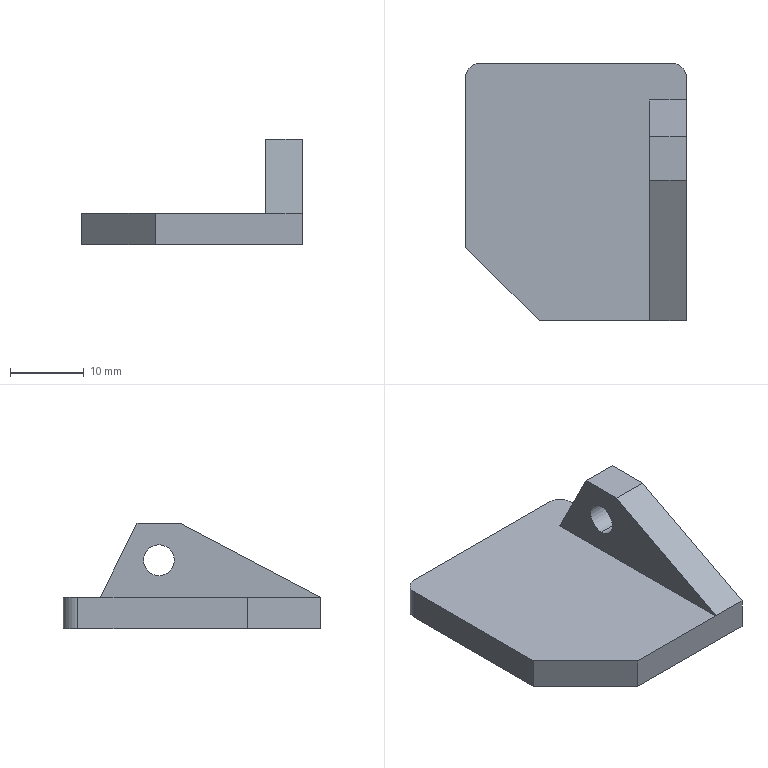Part | SolidWorks | features BaseBody 1 | 1 solid | 15 faces | box 30 x 35 x 14.3 mm | volume 5075 mm3 | plane 11 | cylinder 4 | commonest cylinder face diameters 4 x2 4.2 x2
STEP:
#1=CARTESIAN_POINT('',(269.946,-4053.971,2158.071));
#2=VERTEX_POINT('',#1);
#3=CARTESIAN_POINT('',(269.946,-4053.971,2153.871));
#4=VERTEX_POINT('',#3);
#5=CARTESIAN_POINT('',(269.946,-4053.971,2155.971));
#6=DIRECTION('',(1.,0.,0.));
#7=DIRECTION('',(0.,0.,-1.));
#8=AXIS2_PLACEMENT_3D('',#5,#6,#7);
#9=CIRCLE('',#8,2.1);
#10=EDGE_CURVE('',#2,#4,#9,.T.);
#11=ORIENTED_EDGE('',*,*,#10,.F.);
#12=CARTESIAN_POINT('',(274.946,-4053.971,2158.071));
#13=VERTEX_POINT('',#12);
#14=CARTESIAN_POINT('',(274.946,-4053.971,2158.071));
#15=DIRECTION('',(1.,0.,0.));
#16=VECTOR('',#15,1000.);
#17=LINE('',#14,#16);
#18=EDGE_CURVE('',#2,#13,#17,.T.);
#19=ORIENTED_EDGE('',*,*,#18,.T.);
#20=CARTESIAN_POINT('',(274.946,-4053.971,2153.871));
#21=VERTEX_POINT('',#20);
#22=CARTESIAN_POINT('',(274.946,-4053.971,2155.971));
#23=DIRECTION('',(-1.,0.,0.));
#24=DIRECTION('',(0.,0.,-1.));
#25=AXIS2_PLACEMENT_3D('',#22,#23,#24);
#26=CIRCLE('',#25,2.1);
#27=EDGE_CURVE('',#21,#13,#26,.T.);
#28=ORIENTED_EDGE('',*,*,#27,.F.);
#29=CARTESIAN_POINT('',(274.946,-4053.971,2153.871));
#30=DIRECTION('',(1.,0.,0.));
#31=VECTOR('',#30,1000.);
#32=LINE('',#29,#31);
#33=EDGE_CURVE('',#4,#21,#32,.T.);
#34=ORIENTED_EDGE('',*,*,#33,.F.);
#35=EDGE_LOOP('',(#11,#19,#28,#34));
#36=FACE_OUTER_BOUND('',#35,.T.);
#37=CARTESIAN_POINT('',(274.946,-4053.971,2155.971));
#38=DIRECTION('',(1.,0.,0.));
#39=DIRECTION('',(0.,0.,-1.));
#40=AXIS2_PLACEMENT_3D('',#37,#38,#39);
#41=CYLINDRICAL_SURFACE('',#40,2.1);
#42=ADVANCED_FACE('',(#36),#41,.F.);
#43=CARTESIAN_POINT('',(272.946,-4040.971,2146.671));
#44=VERTEX_POINT('',#43);
#45=CARTESIAN_POINT('',(246.946,-4040.971,2146.671));
#46=VERTEX_POINT('',#45);
#47=CARTESIAN_POINT('',(254.946,-4040.971,2146.671));
#48=DIRECTION('',(-1.,0.,0.));
#49=VECTOR('',#48,1000.);
#50=LINE('',#47,#49);
#51=EDGE_CURVE('',#44,#46,#50,.T.);
#52=ORIENTED_EDGE('',*,*,#51,.F.);
#53=CARTESIAN_POINT('',(274.946,-4042.971,2146.671));
#54=VERTEX_POINT('',#53);
#55=CARTESIAN_POINT('',(272.946,-4042.971,2146.671));
#56=DIRECTION('',(0.,0.,1.));
#57=DIRECTION('',(1.,0.,0.));
#58=AXIS2_PLACEMENT_3D('',#55,#56,#57);
#59=CIRCLE('',#58,2.);
#60=EDGE_CURVE('',#54,#44,#59,.T.);
#61=ORIENTED_EDGE('',*,*,#60,.F.);
#62=CARTESIAN_POINT('',(274.946,-4075.971,2146.671));
#63=VERTEX_POINT('',#62);
#64=CARTESIAN_POINT('',(274.946,-4075.971,2146.671));
#65=DIRECTION('',(0.,1.,0.));
#66=VECTOR('',#65,1000.);
#67=LINE('',#64,#66);
#68=EDGE_CURVE('',#63,#54,#67,.T.);
#69=ORIENTED_EDGE('',*,*,#68,.F.);
#70=CARTESIAN_POINT('',(254.946,-4075.971,2146.671));
#71=VERTEX_POINT('',#70);
#72=CARTESIAN_POINT('',(254.946,-4075.971,2146.671));
#73=DIRECTION('',(1.,0.,0.));
#74=VECTOR('',#73,1000.);
#75=LINE('',#72,#74);
#76=EDGE_CURVE('',#71,#63,#75,.T.);
#77=ORIENTED_EDGE('',*,*,#76,.F.);
#78=CARTESIAN_POINT('',(244.946,-4065.971,2146.671));
#79=VERTEX_POINT('',#78);
#80=CARTESIAN_POINT('',(244.946,-4065.971,2146.671));
#81=DIRECTION('',(0.7071,-0.7071,0.));
#82=VECTOR('',#81,1000.);
#83=LINE('',#80,#82);
#84=EDGE_CURVE('',#79,#71,#83,.T.);
#85=ORIENTED_EDGE('',*,*,#84,.F.);
#86=CARTESIAN_POINT('',(244.946,-4042.971,2146.671));
#87=VERTEX_POINT('',#86);
#88=CARTESIAN_POINT('',(244.946,-4075.971,2146.671));
#89=DIRECTION('',(0.,-1.,0.));
#90=VECTOR('',#89,1000.);
#91=LINE('',#88,#90);
#92=EDGE_CURVE('',#87,#79,#91,.T.);
#93=ORIENTED_EDGE('',*,*,#92,.F.);
#94=CARTESIAN_POINT('',(246.946,-4042.971,2146.671));
#95=DIRECTION('',(0.,0.,1.));
#96=DIRECTION('',(1.,0.,0.));
#97=AXIS2_PLACEMENT_3D('',#94,#95,#96);
#98=CIRCLE('',#97,2.);
#99=EDGE_CURVE('',#46,#87,#98,.T.);
#100=ORIENTED_EDGE('',*,*,#99,.F.);
#101=EDGE_LOOP('',(#52,#61,#69,#77,#85,#93,#100));
#102=FACE_OUTER_BOUND('',#101,.T.);
#103=CARTESIAN_POINT('',(254.946,-4075.971,2146.671));
#104=DIRECTION('',(0.,0.,1.));
#105=DIRECTION('',(0.,-1.,0.));
#106=AXIS2_PLACEMENT_3D('',#103,#104,#105);
#107=PLANE('',#106);
#108=ADVANCED_FACE('',(#102),#107,.F.);
#109=CARTESIAN_POINT('',(244.946,-4042.971,2150.921));
#110=VERTEX_POINT('',#109);
#111=CARTESIAN_POINT('',(244.946,-4042.971,2150.921));
#112=DIRECTION('',(0.,0.,1.));
#113=VECTOR('',#112,1000.);
#114=LINE('',#111,#113);
#115=EDGE_CURVE('',#87,#110,#114,.T.);
#116=ORIENTED_EDGE('',*,*,#115,.T.);
#117=CARTESIAN_POINT('',(246.946,-4040.971,2150.921));
#118=VERTEX_POINT('',#117);
#119=CARTESIAN_POINT('',(246.946,-4042.971,2150.921));
#120=DIRECTION('',(0.,0.,-1.));
#121=DIRECTION('',(1.,0.,0.));
#122=AXIS2_PLACEMENT_3D('',#119,#120,#121);
#123=CIRCLE('',#122,2.);
#124=EDGE_CURVE('',#110,#118,#123,.T.);
#125=ORIENTED_EDGE('',*,*,#124,.T.);
#126=CARTESIAN_POINT('',(246.946,-4040.971,2150.921));
#127=DIRECTION('',(0.,0.,-1.));
#128=VECTOR('',#127,1000.);
#129=LINE('',#126,#128);
#130=EDGE_CURVE('',#118,#46,#129,.T.);
#131=ORIENTED_EDGE('',*,*,#130,.T.);
#132=ORIENTED_EDGE('',*,*,#99,.T.);
#133=EDGE_LOOP('',(#116,#125,#131,#132));
#134=FACE_OUTER_BOUND('',#133,.T.);
#135=CARTESIAN_POINT('',(246.946,-4042.971,2150.921));
#136=DIRECTION('',(0.,0.,1.));
#137=DIRECTION('',(1.,0.,0.));
#138=AXIS2_PLACEMENT_3D('',#135,#136,#137);
#139=CYLINDRICAL_SURFACE('',#138,2.);
#140=ADVANCED_FACE('',(#134),#139,.T.);
#141=ORIENTED_EDGE('',*,*,#130,.F.);
#142=CARTESIAN_POINT('',(272.946,-4040.971,2150.921));
#143=VERTEX_POINT('',#142);
#144=CARTESIAN_POINT('',(244.946,-4040.971,2150.921));
#145=DIRECTION('',(1.,0.,0.));
#146=VECTOR('',#145,1000.);
#147=LINE('',#144,#146);
#148=EDGE_CURVE('',#118,#143,#147,.T.);
#149=ORIENTED_EDGE('',*,*,#148,.T.);
#150=CARTESIAN_POINT('',(272.946,-4040.971,2150.921));
#151=DIRECTION('',(0.,0.,-1.));
#152=VECTOR('',#151,1000.);
#153=LINE('',#150,#152);
#154=EDGE_CURVE('',#143,#44,#153,.T.);
#155=ORIENTED_EDGE('',*,*,#154,.T.);
#156=ORIENTED_EDGE('',*,*,#51,.T.);
#157=EDGE_LOOP('',(#141,#149,#155,#156));
#158=FACE_OUTER_BOUND('',#157,.T.);
#159=CARTESIAN_POINT('',(244.946,-4040.971,2150.921));
#160=DIRECTION('',(0.,1.,0.));
#161=DIRECTION('',(0.,0.,1.));
#162=AXIS2_PLACEMENT_3D('',#159,#160,#161);
#163=PLANE('',#162);
#164=ADVANCED_FACE('',(#158),#163,.T.);
#165=ORIENTED_EDGE('',*,*,#154,.F.);
#166=CARTESIAN_POINT('',(274.946,-4042.971,2150.921));
#167=VERTEX_POINT('',#166);
#168=CARTESIAN_POINT('',(272.946,-4042.971,2150.921));
#169=DIRECTION('',(0.,0.,-1.));
#170=DIRECTION('',(1.,0.,0.));
#171=AXIS2_PLACEMENT_3D('',#168,#169,#170);
#172=CIRCLE('',#171,2.);
#173=EDGE_CURVE('',#143,#167,#172,.T.);
#174=ORIENTED_EDGE('',*,*,#173,.T.);
#175=CARTESIAN_POINT('',(274.946,-4042.971,2150.921));
#176=DIRECTION('',(0.,0.,-1.));
#177=VECTOR('',#176,1000.);
#178=LINE('',#175,#177);
#179=EDGE_CURVE('',#167,#54,#178,.T.);
#180=ORIENTED_EDGE('',*,*,#179,.T.);
#181=ORIENTED_EDGE('',*,*,#60,.T.);
#182=EDGE_LOOP('',(#165,#174,#180,#181));
#183=FACE_OUTER_BOUND('',#182,.T.);
#184=CARTESIAN_POINT('',(272.946,-4042.971,2150.921));
#185=DIRECTION('',(0.,0.,1.));
#186=DIRECTION('',(1.,0.,0.));
#187=AXIS2_PLACEMENT_3D('',#184,#185,#186);
#188=CYLINDRICAL_SURFACE('',#187,2.);
#189=ADVANCED_FACE('',(#183),#188,.T.);
#190=CARTESIAN_POINT('',(274.946,-4075.971,2150.921));
#191=VERTEX_POINT('',#190);
#192=CARTESIAN_POINT('',(274.946,-4075.971,2150.921));
#193=DIRECTION('',(0.,0.,-1.));
#194=VECTOR('',#193,1000.);
#195=LINE('',#192,#194);
#196=EDGE_CURVE('',#191,#63,#195,.T.);
#197=ORIENTED_EDGE('',*,*,#196,.T.);
#198=ORIENTED_EDGE('',*,*,#68,.T.);
#199=ORIENTED_EDGE('',*,*,#179,.F.);
#200=CARTESIAN_POINT('',(274.946,-4045.971,2150.921));
#201=VERTEX_POINT('',#200);
#202=CARTESIAN_POINT('',(274.946,-4040.971,2150.921));
#203=DIRECTION('',(0.,-1.,0.));
#204=VECTOR('',#203,1000.);
#205=LINE('',#202,#204);
#206=EDGE_CURVE('',#167,#201,#205,.T.);
#207=ORIENTED_EDGE('',*,*,#206,.T.);
#208=CARTESIAN_POINT('',(274.946,-4050.996,2160.971));
#209=VERTEX_POINT('',#208);
#210=CARTESIAN_POINT('',(274.946,-4045.971,2150.921));
#211=DIRECTION('',(0.,-0.4472,0.8944));
#212=VECTOR('',#211,1000.);
#213=LINE('',#210,#212);
#214=EDGE_CURVE('',#201,#209,#213,.T.);
#215=ORIENTED_EDGE('',*,*,#214,.T.);
#216=CARTESIAN_POINT('',(274.946,-4056.876,2160.971));
#217=VERTEX_POINT('',#216);
#218=CARTESIAN_POINT('',(274.946,-4040.971,2160.971));
#219=DIRECTION('',(0.,-1.,0.));
#220=VECTOR('',#219,1000.);
#221=LINE('',#218,#220);
#222=EDGE_CURVE('',#209,#217,#221,.T.);
#223=ORIENTED_EDGE('',*,*,#222,.T.);
#224=CARTESIAN_POINT('',(274.946,-4056.876,2160.971));
#225=DIRECTION('',(0.,-0.8849,-0.4657));
#226=VECTOR('',#225,1000.);
#227=LINE('',#224,#226);
#228=EDGE_CURVE('',#217,#191,#227,.T.);
#229=ORIENTED_EDGE('',*,*,#228,.T.);
#230=EDGE_LOOP('',(#197,#198,#199,#207,#215,#223,#229));
#231=FACE_OUTER_BOUND('',#230,.T.);
#232=ORIENTED_EDGE('',*,*,#27,.T.);
#233=CARTESIAN_POINT('',(274.946,-4053.971,2155.971));
#234=DIRECTION('',(-1.,0.,0.));
#235=DIRECTION('',(0.,0.,-1.));
#236=AXIS2_PLACEMENT_3D('',#233,#234,#235);
#237=CIRCLE('',#236,2.1);
#238=EDGE_CURVE('',#13,#21,#237,.T.);
#239=ORIENTED_EDGE('',*,*,#238,.T.);
#240=EDGE_LOOP('',(#232,#239));
#241=FACE_BOUND('',#240,.T.);
#242=CARTESIAN_POINT('',(274.946,-4040.971,2150.921));
#243=DIRECTION('',(1.,0.,0.));
#244=DIRECTION('',(0.,1.,0.));
#245=AXIS2_PLACEMENT_3D('',#242,#243,#244);
#246=PLANE('',#245);
#247=ADVANCED_FACE('',(#231,#241),#246,.T.);
#248=CARTESIAN_POINT('',(269.946,-4075.971,2150.921));
#249=VERTEX_POINT('',#248);
#250=CARTESIAN_POINT('',(274.946,-4075.971,2150.921));
#251=DIRECTION('',(-1.,0.,0.));
#252=VECTOR('',#251,1000.);
#253=LINE('',#250,#252);
#254=EDGE_CURVE('',#191,#249,#253,.T.);
#255=ORIENTED_EDGE('',*,*,#254,.T.);
#256=CARTESIAN_POINT('',(254.946,-4075.971,2150.921));
#257=VERTEX_POINT('',#256);
#258=CARTESIAN_POINT('',(274.946,-4075.971,2150.921));
#259=DIRECTION('',(-1.,0.,0.));
#260=VECTOR('',#259,1000.);
#261=LINE('',#258,#260);
#262=EDGE_CURVE('',#249,#257,#261,.T.);
#263=ORIENTED_EDGE('',*,*,#262,.T.);
#264=CARTESIAN_POINT('',(254.946,-4075.971,2150.921));
#265=DIRECTION('',(0.,0.,-1.));
#266=VECTOR('',#265,1000.);
#267=LINE('',#264,#266);
#268=EDGE_CURVE('',#257,#71,#267,.T.);
#269=ORIENTED_EDGE('',*,*,#268,.T.);
#270=ORIENTED_EDGE('',*,*,#76,.T.);
#271=ORIENTED_EDGE('',*,*,#196,.F.);
#272=EDGE_LOOP('',(#255,#263,#269,#270,#271));
#273=FACE_OUTER_BOUND('',#272,.T.);
#274=CARTESIAN_POINT('',(274.946,-4075.971,2150.921));
#275=DIRECTION('',(0.,-1.,0.));
#276=DIRECTION('',(0.,0.,-1.));
#277=AXIS2_PLACEMENT_3D('',#274,#275,#276);
#278=PLANE('',#277);
#279=ADVANCED_FACE('',(#273),#278,.T.);
#280=ORIENTED_EDGE('',*,*,#268,.F.);
#281=CARTESIAN_POINT('',(244.946,-4065.971,2150.921));
#282=VERTEX_POINT('',#281);
#283=CARTESIAN_POINT('',(254.946,-4075.971,2150.921));
#284=DIRECTION('',(-0.7071,0.7071,0.));
#285=VECTOR('',#284,1000.);
#286=LINE('',#283,#285);
#287=EDGE_CURVE('',#257,#282,#286,.T.);
#288=ORIENTED_EDGE('',*,*,#287,.T.);
#289=CARTESIAN_POINT('',(244.946,-4065.971,2150.921));
#290=DIRECTION('',(0.,0.,-1.));
#291=VECTOR('',#290,1000.);
#292=LINE('',#289,#291);
#293=EDGE_CURVE('',#282,#79,#292,.T.);
#294=ORIENTED_EDGE('',*,*,#293,.T.);
#295=ORIENTED_EDGE('',*,*,#84,.T.);
#296=EDGE_LOOP('',(#280,#288,#294,#295));
#297=FACE_OUTER_BOUND('',#296,.T.);
#298=CARTESIAN_POINT('',(254.946,-4075.971,2150.921));
#299=DIRECTION('',(-0.7071,-0.7071,0.));
#300=DIRECTION('',(0.7071,-0.7071,0.));
#301=AXIS2_PLACEMENT_3D('',#298,#299,#300);
#302=PLANE('',#301);
#303=ADVANCED_FACE('',(#297),#302,.T.);
#304=ORIENTED_EDGE('',*,*,#293,.F.);
#305=CARTESIAN_POINT('',(244.946,-4065.971,2150.921));
#306=DIRECTION('',(0.,1.,0.));
#307=VECTOR('',#306,1000.);
#308=LINE('',#305,#307);
#309=EDGE_CURVE('',#282,#110,#308,.T.);
#310=ORIENTED_EDGE('',*,*,#309,.T.);
#311=ORIENTED_EDGE('',*,*,#115,.F.);
#312=ORIENTED_EDGE('',*,*,#92,.T.);
#313=EDGE_LOOP('',(#304,#310,#311,#312));
#314=FACE_OUTER_BOUND('',#313,.T.);
#315=CARTESIAN_POINT('',(244.946,-4065.971,2150.921));
#316=DIRECTION('',(-1.,0.,0.));
#317=DIRECTION('',(0.,-1.,0.));
#318=AXIS2_PLACEMENT_3D('',#315,#316,#317);
#319=PLANE('',#318);
#320=ADVANCED_FACE('',(#314),#319,.T.);
#321=ORIENTED_EDGE('',*,*,#287,.F.);
#322=ORIENTED_EDGE('',*,*,#262,.F.);
#323=CARTESIAN_POINT('',(269.946,-4045.971,2150.921));
#324=VERTEX_POINT('',#323);
#325=CARTESIAN_POINT('',(269.946,-4059.971,2150.921));
#326=DIRECTION('',(0.,1.,0.));
#327=VECTOR('',#326,1000.);
#328=LINE('',#325,#327);
#329=EDGE_CURVE('',#249,#324,#328,.T.);
#330=ORIENTED_EDGE('',*,*,#329,.T.);
#331=CARTESIAN_POINT('',(258.946,-4045.971,2150.921));
#332=DIRECTION('',(1.,0.,0.));
#333=VECTOR('',#332,1000.);
#334=LINE('',#331,#333);
#335=EDGE_CURVE('',#324,#201,#334,.T.);
#336=ORIENTED_EDGE('',*,*,#335,.T.);
#337=ORIENTED_EDGE('',*,*,#206,.F.);
#338=ORIENTED_EDGE('',*,*,#173,.F.);
#339=ORIENTED_EDGE('',*,*,#148,.F.);
#340=ORIENTED_EDGE('',*,*,#124,.F.);
#341=ORIENTED_EDGE('',*,*,#309,.F.);
#342=EDGE_LOOP('',(#321,#322,#330,#336,#337,#338,#339,#340,#341));
#343=FACE_OUTER_BOUND('',#342,.T.);
#344=CARTESIAN_POINT('',(258.946,-4059.971,2150.921));
#345=DIRECTION('',(0.,0.,1.));
#346=DIRECTION('',(0.,-1.,0.));
#347=AXIS2_PLACEMENT_3D('',#344,#345,#346);
#348=PLANE('',#347);
#349=ADVANCED_FACE('',(#343),#348,.T.);
#350=ORIENTED_EDGE('',*,*,#228,.F.);
#351=CARTESIAN_POINT('',(269.946,-4056.876,2160.971));
#352=VERTEX_POINT('',#351);
#353=CARTESIAN_POINT('',(274.946,-4056.876,2160.971));
#354=DIRECTION('',(-1.,0.,0.));
#355=VECTOR('',#354,1000.);
#356=LINE('',#353,#355);
#357=EDGE_CURVE('',#217,#352,#356,.T.);
#358=ORIENTED_EDGE('',*,*,#357,.T.);
#359=CARTESIAN_POINT('',(269.946,-4075.971,2150.921));
#360=DIRECTION('',(0.,-0.8849,-0.4657));
#361=VECTOR('',#360,1000.);
#362=LINE('',#359,#361);
#363=EDGE_CURVE('',#352,#249,#362,.T.);
#364=ORIENTED_EDGE('',*,*,#363,.T.);
#365=ORIENTED_EDGE('',*,*,#254,.F.);
#366=EDGE_LOOP('',(#350,#358,#364,#365));
#367=FACE_OUTER_BOUND('',#366,.T.);
#368=CARTESIAN_POINT('',(274.946,-4075.971,2150.921));
#369=DIRECTION('',(0.,-0.4657,0.8849));
#370=DIRECTION('',(0.,-0.8849,-0.4657));
#371=AXIS2_PLACEMENT_3D('',#368,#369,#370);
#372=PLANE('',#371);
#373=ADVANCED_FACE('',(#367),#372,.T.);
#374=ORIENTED_EDGE('',*,*,#222,.F.);
#375=CARTESIAN_POINT('',(269.946,-4050.996,2160.971));
#376=VERTEX_POINT('',#375);
#377=CARTESIAN_POINT('',(274.946,-4050.996,2160.971));
#378=DIRECTION('',(-1.,0.,0.));
#379=VECTOR('',#378,1000.);
#380=LINE('',#377,#379);
#381=EDGE_CURVE('',#209,#376,#380,.T.);
#382=ORIENTED_EDGE('',*,*,#381,.T.);
#383=CARTESIAN_POINT('',(269.946,-4056.971,2160.971));
#384=DIRECTION('',(0.,-1.,0.));
#385=VECTOR('',#384,1000.);
#386=LINE('',#383,#385);
#387=EDGE_CURVE('',#376,#352,#386,.T.);
#388=ORIENTED_EDGE('',*,*,#387,.T.);
#389=ORIENTED_EDGE('',*,*,#357,.F.);
#390=EDGE_LOOP('',(#374,#382,#388,#389));
#391=FACE_OUTER_BOUND('',#390,.T.);
#392=CARTESIAN_POINT('',(274.946,-4056.971,2160.971));
#393=DIRECTION('',(0.,0.,1.));
#394=DIRECTION('',(0.,-1.,0.));
#395=AXIS2_PLACEMENT_3D('',#392,#393,#394);
#396=PLANE('',#395);
#397=ADVANCED_FACE('',(#391),#396,.T.);
#398=ORIENTED_EDGE('',*,*,#214,.F.);
#399=ORIENTED_EDGE('',*,*,#335,.F.);
#400=CARTESIAN_POINT('',(269.946,-4050.971,2160.921));
#401=DIRECTION('',(0.,-0.4472,0.8944));
#402=VECTOR('',#401,1000.);
#403=LINE('',#400,#402);
#404=EDGE_CURVE('',#324,#376,#403,.T.);
#405=ORIENTED_EDGE('',*,*,#404,.T.);
#406=ORIENTED_EDGE('',*,*,#381,.F.);
#407=EDGE_LOOP('',(#398,#399,#405,#406));
#408=FACE_OUTER_BOUND('',#407,.T.);
#409=CARTESIAN_POINT('',(274.946,-4050.971,2160.921));
#410=DIRECTION('',(0.,0.8944,0.4472));
#411=DIRECTION('',(0.,-0.4472,0.8944));
#412=AXIS2_PLACEMENT_3D('',#409,#410,#411);
#413=PLANE('',#412);
#414=ADVANCED_FACE('',(#408),#413,.T.);
#415=ORIENTED_EDGE('',*,*,#18,.F.);
#416=CARTESIAN_POINT('',(269.946,-4053.971,2155.971));
#417=DIRECTION('',(1.,0.,0.));
#418=DIRECTION('',(0.,0.,-1.));
#419=AXIS2_PLACEMENT_3D('',#416,#417,#418);
#420=CIRCLE('',#419,2.1);
#421=EDGE_CURVE('',#4,#2,#420,.T.);
#422=ORIENTED_EDGE('',*,*,#421,.F.);
#423=ORIENTED_EDGE('',*,*,#33,.T.);
#424=ORIENTED_EDGE('',*,*,#238,.F.);
#425=EDGE_LOOP('',(#415,#422,#423,#424));
#426=FACE_OUTER_BOUND('',#425,.T.);
#427=CARTESIAN_POINT('',(274.946,-4053.971,2155.971));
#428=DIRECTION('',(1.,0.,0.));
#429=DIRECTION('',(0.,0.,-1.));
#430=AXIS2_PLACEMENT_3D('',#427,#428,#429);
#431=CYLINDRICAL_SURFACE('',#430,2.1);
#432=ADVANCED_FACE('',(#426),#431,.F.);
#433=ORIENTED_EDGE('',*,*,#404,.F.);
#434=ORIENTED_EDGE('',*,*,#329,.F.);
#435=ORIENTED_EDGE('',*,*,#363,.F.);
#436=ORIENTED_EDGE('',*,*,#387,.F.);
#437=EDGE_LOOP('',(#433,#434,#435,#436));
#438=FACE_OUTER_BOUND('',#437,.T.);
#439=ORIENTED_EDGE('',*,*,#421,.T.);
#440=ORIENTED_EDGE('',*,*,#10,.T.);
#441=EDGE_LOOP('',(#439,#440));
#442=FACE_BOUND('',#441,.T.);
#443=CARTESIAN_POINT('',(269.946,-4056.971,2160.921));
#444=DIRECTION('',(1.,0.,0.));
#445=DIRECTION('',(0.,0.,-1.));
#446=AXIS2_PLACEMENT_3D('',#443,#444,#445);
#447=PLANE('',#446);
#448=ADVANCED_FACE('',(#438,#442),#447,.F.);
#449=CLOSED_SHELL('',(#42,#108,#140,#164,#189,#247,#279,#303,#320,#349,#373,#397,#414,#432,#448));
#450=MANIFOLD_SOLID_BREP('',#449);
#451=CARTESIAN_POINT('',(0.,0.,0.));
#452=DIRECTION('',(0.,0.,1.));
#453=DIRECTION('',(1.,0.,0.));
#454=AXIS2_PLACEMENT_3D('',#451,#452,#453);
#455=(LENGTH_UNIT()NAMED_UNIT(*)SI_UNIT(.MILLI.,.METRE.));
#456=UNCERTAINTY_MEASURE_WITH_UNIT(LENGTH_MEASURE(0.00001),#455,'','');
#457=(NAMED_UNIT(*)PLANE_ANGLE_UNIT()SI_UNIT($,.RADIAN.));
#458=(NAMED_UNIT(*)SI_UNIT($,.STERADIAN.)SOLID_ANGLE_UNIT());
#459=(GEOMETRIC_REPRESENTATION_CONTEXT(3)GLOBAL_UNCERTAINTY_ASSIGNED_CONTEXT((#456))GLOBAL_UNIT_ASSIGNED_CONTEXT((#455,#457,#458))REPRESENTATION_CONTEXT('',''));
#460=ADVANCED_BREP_SHAPE_REPRESENTATION('',(#450,#454),#459);